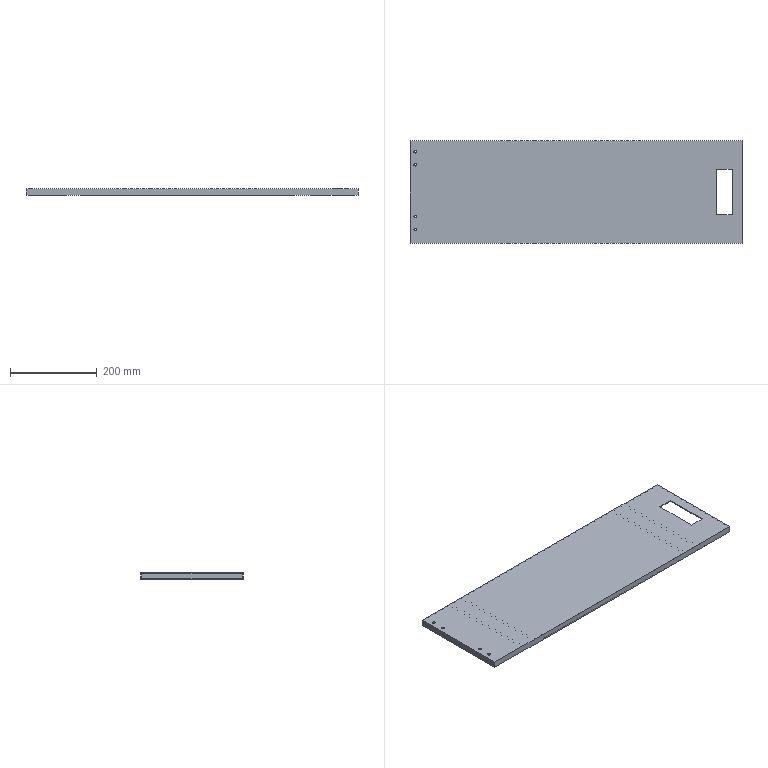Part | STEP file | Rear upper door | 1 solid | 70 faces | box 767 x 237 x 15 mm | volume 502024 mm3 | plane 58 | cylinder 12 | commonest cylinder face diameters 6.2 x12